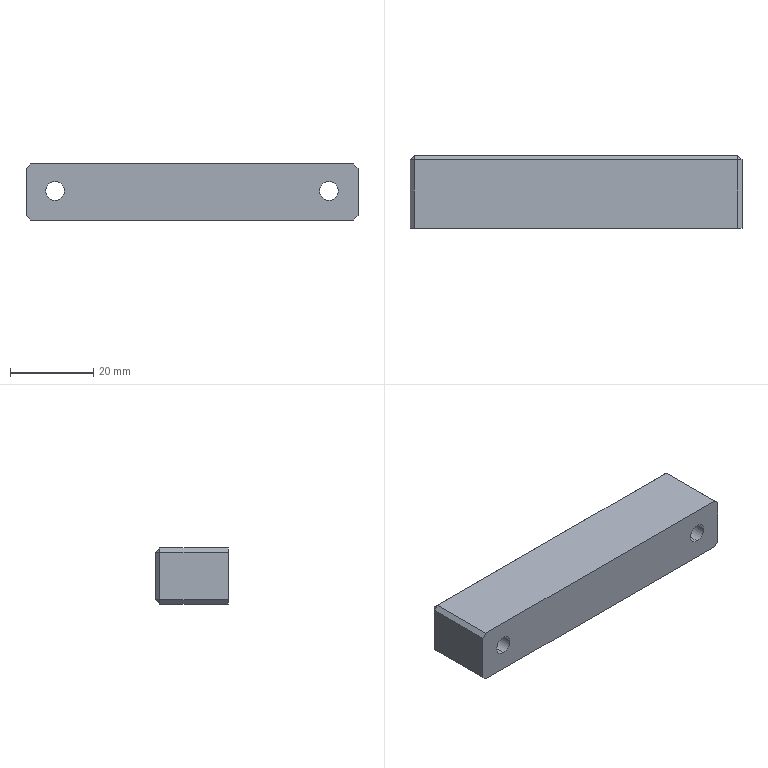Part | STEP file | 229H151426 Default | 1 solid | 28 faces | box 80 x 17.5 x 13.5 mm | volume 17874 mm3 | plane 20 | cylinder 8 | commonest cylinder face diameters 4.5 x4 8 x4
STEP:
#1=CARTESIAN_POINT('',(-33.,3.75,3.));
#2=VERTEX_POINT('',#1);
#3=CARTESIAN_POINT('',(-33.,3.75,11.));
#4=VERTEX_POINT('',#3);
#5=CARTESIAN_POINT('',(-33.,3.75,7.));
#6=DIRECTION('',(0.,1.,0.));
#7=DIRECTION('',(0.,0.,1.));
#8=AXIS2_PLACEMENT_3D('',#5,#6,#7);
#9=CIRCLE('',#8,4.);
#10=EDGE_CURVE('',#2,#4,#9,.T.);
#11=ORIENTED_EDGE('',*,*,#10,.F.);
#12=CARTESIAN_POINT('',(-33.,8.75,3.));
#13=VERTEX_POINT('',#12);
#14=CARTESIAN_POINT('',(-33.,8.75,3.));
#15=DIRECTION('',(0.,1.,0.));
#16=VECTOR('',#15,1000.);
#17=LINE('',#14,#16);
#18=EDGE_CURVE('',#2,#13,#17,.T.);
#19=ORIENTED_EDGE('',*,*,#18,.T.);
#20=CARTESIAN_POINT('',(-33.,8.75,11.));
#21=VERTEX_POINT('',#20);
#22=CARTESIAN_POINT('',(-33.,8.75,7.));
#23=DIRECTION('',(0.,1.,0.));
#24=DIRECTION('',(0.,0.,1.));
#25=AXIS2_PLACEMENT_3D('',#22,#23,#24);
#26=CIRCLE('',#25,4.);
#27=EDGE_CURVE('',#13,#21,#26,.T.);
#28=ORIENTED_EDGE('',*,*,#27,.T.);
#29=CARTESIAN_POINT('',(-33.,8.75,11.));
#30=DIRECTION('',(0.,1.,0.));
#31=VECTOR('',#30,1000.);
#32=LINE('',#29,#31);
#33=EDGE_CURVE('',#4,#21,#32,.T.);
#34=ORIENTED_EDGE('',*,*,#33,.F.);
#35=EDGE_LOOP('',(#11,#19,#28,#34));
#36=FACE_OUTER_BOUND('',#35,.T.);
#37=CARTESIAN_POINT('',(-33.,8.75,7.));
#38=DIRECTION('',(0.,1.,0.));
#39=DIRECTION('',(0.,0.,1.));
#40=AXIS2_PLACEMENT_3D('',#37,#38,#39);
#41=CYLINDRICAL_SURFACE('',#40,4.);
#42=ADVANCED_FACE('',(#36),#41,.F.);
#43=CARTESIAN_POINT('',(-33.,-8.75,4.75));
#44=VERTEX_POINT('',#43);
#45=CARTESIAN_POINT('',(-33.,-8.75,9.25));
#46=VERTEX_POINT('',#45);
#47=CARTESIAN_POINT('',(-33.,-8.75,7.));
#48=DIRECTION('',(0.,1.,0.));
#49=DIRECTION('',(0.,0.,1.));
#50=AXIS2_PLACEMENT_3D('',#47,#48,#49);
#51=CIRCLE('',#50,2.25);
#52=EDGE_CURVE('',#44,#46,#51,.T.);
#53=ORIENTED_EDGE('',*,*,#52,.F.);
#54=CARTESIAN_POINT('',(-33.,3.75,4.75));
#55=VERTEX_POINT('',#54);
#56=CARTESIAN_POINT('',(-33.,8.75,4.75));
#57=DIRECTION('',(0.,1.,0.));
#58=VECTOR('',#57,1000.);
#59=LINE('',#56,#58);
#60=EDGE_CURVE('',#44,#55,#59,.T.);
#61=ORIENTED_EDGE('',*,*,#60,.T.);
#62=CARTESIAN_POINT('',(-33.,3.75,9.25));
#63=VERTEX_POINT('',#62);
#64=CARTESIAN_POINT('',(-33.,3.75,7.));
#65=DIRECTION('',(0.,1.,0.));
#66=DIRECTION('',(0.,0.,1.));
#67=AXIS2_PLACEMENT_3D('',#64,#65,#66);
#68=CIRCLE('',#67,2.25);
#69=EDGE_CURVE('',#55,#63,#68,.T.);
#70=ORIENTED_EDGE('',*,*,#69,.T.);
#71=CARTESIAN_POINT('',(-33.,8.75,9.25));
#72=DIRECTION('',(0.,1.,0.));
#73=VECTOR('',#72,1000.);
#74=LINE('',#71,#73);
#75=EDGE_CURVE('',#46,#63,#74,.T.);
#76=ORIENTED_EDGE('',*,*,#75,.F.);
#77=EDGE_LOOP('',(#53,#61,#70,#76));
#78=FACE_OUTER_BOUND('',#77,.T.);
#79=CARTESIAN_POINT('',(-33.,8.75,7.));
#80=DIRECTION('',(0.,1.,0.));
#81=DIRECTION('',(0.,0.,1.));
#82=AXIS2_PLACEMENT_3D('',#79,#80,#81);
#83=CYLINDRICAL_SURFACE('',#82,2.25);
#84=ADVANCED_FACE('',(#78),#83,.F.);
#85=CARTESIAN_POINT('',(33.,3.75,3.));
#86=VERTEX_POINT('',#85);
#87=CARTESIAN_POINT('',(33.,3.75,11.));
#88=VERTEX_POINT('',#87);
#89=CARTESIAN_POINT('',(33.,3.75,7.));
#90=DIRECTION('',(0.,1.,0.));
#91=DIRECTION('',(0.,0.,1.));
#92=AXIS2_PLACEMENT_3D('',#89,#90,#91);
#93=CIRCLE('',#92,4.);
#94=EDGE_CURVE('',#86,#88,#93,.T.);
#95=ORIENTED_EDGE('',*,*,#94,.F.);
#96=CARTESIAN_POINT('',(33.,8.75,3.));
#97=VERTEX_POINT('',#96);
#98=CARTESIAN_POINT('',(33.,8.75,3.));
#99=DIRECTION('',(0.,1.,0.));
#100=VECTOR('',#99,1000.);
#101=LINE('',#98,#100);
#102=EDGE_CURVE('',#86,#97,#101,.T.);
#103=ORIENTED_EDGE('',*,*,#102,.T.);
#104=CARTESIAN_POINT('',(33.,8.75,11.));
#105=VERTEX_POINT('',#104);
#106=CARTESIAN_POINT('',(33.,8.75,7.));
#107=DIRECTION('',(0.,1.,0.));
#108=DIRECTION('',(0.,0.,1.));
#109=AXIS2_PLACEMENT_3D('',#106,#107,#108);
#110=CIRCLE('',#109,4.);
#111=EDGE_CURVE('',#97,#105,#110,.T.);
#112=ORIENTED_EDGE('',*,*,#111,.T.);
#113=CARTESIAN_POINT('',(33.,8.75,11.));
#114=DIRECTION('',(0.,1.,0.));
#115=VECTOR('',#114,1000.);
#116=LINE('',#113,#115);
#117=EDGE_CURVE('',#88,#105,#116,.T.);
#118=ORIENTED_EDGE('',*,*,#117,.F.);
#119=EDGE_LOOP('',(#95,#103,#112,#118));
#120=FACE_OUTER_BOUND('',#119,.T.);
#121=CARTESIAN_POINT('',(33.,8.75,7.));
#122=DIRECTION('',(0.,1.,0.));
#123=DIRECTION('',(0.,0.,1.));
#124=AXIS2_PLACEMENT_3D('',#121,#122,#123);
#125=CYLINDRICAL_SURFACE('',#124,4.);
#126=ADVANCED_FACE('',(#120),#125,.F.);
#127=CARTESIAN_POINT('',(33.,-8.75,4.75));
#128=VERTEX_POINT('',#127);
#129=CARTESIAN_POINT('',(33.,-8.75,9.25));
#130=VERTEX_POINT('',#129);
#131=CARTESIAN_POINT('',(33.,-8.75,7.));
#132=DIRECTION('',(0.,1.,0.));
#133=DIRECTION('',(0.,0.,1.));
#134=AXIS2_PLACEMENT_3D('',#131,#132,#133);
#135=CIRCLE('',#134,2.25);
#136=EDGE_CURVE('',#128,#130,#135,.T.);
#137=ORIENTED_EDGE('',*,*,#136,.F.);
#138=CARTESIAN_POINT('',(33.,3.75,4.75));
#139=VERTEX_POINT('',#138);
#140=CARTESIAN_POINT('',(33.,8.75,4.75));
#141=DIRECTION('',(0.,1.,0.));
#142=VECTOR('',#141,1000.);
#143=LINE('',#140,#142);
#144=EDGE_CURVE('',#128,#139,#143,.T.);
#145=ORIENTED_EDGE('',*,*,#144,.T.);
#146=CARTESIAN_POINT('',(33.,3.75,9.25));
#147=VERTEX_POINT('',#146);
#148=CARTESIAN_POINT('',(33.,3.75,7.));
#149=DIRECTION('',(0.,1.,0.));
#150=DIRECTION('',(0.,0.,1.));
#151=AXIS2_PLACEMENT_3D('',#148,#149,#150);
#152=CIRCLE('',#151,2.25);
#153=EDGE_CURVE('',#139,#147,#152,.T.);
#154=ORIENTED_EDGE('',*,*,#153,.T.);
#155=CARTESIAN_POINT('',(33.,8.75,9.25));
#156=DIRECTION('',(0.,1.,0.));
#157=VECTOR('',#156,1000.);
#158=LINE('',#155,#157);
#159=EDGE_CURVE('',#130,#147,#158,.T.);
#160=ORIENTED_EDGE('',*,*,#159,.F.);
#161=EDGE_LOOP('',(#137,#145,#154,#160));
#162=FACE_OUTER_BOUND('',#161,.T.);
#163=CARTESIAN_POINT('',(33.,8.75,7.));
#164=DIRECTION('',(0.,1.,0.));
#165=DIRECTION('',(0.,0.,1.));
#166=AXIS2_PLACEMENT_3D('',#163,#164,#165);
#167=CYLINDRICAL_SURFACE('',#166,2.25);
#168=ADVANCED_FACE('',(#162),#167,.F.);
#169=CARTESIAN_POINT('',(40.,-8.75,12.5));
#170=VERTEX_POINT('',#169);
#171=CARTESIAN_POINT('',(40.,-8.75,1.));
#172=VERTEX_POINT('',#171);
#173=CARTESIAN_POINT('',(40.,-8.75,13.5));
#174=DIRECTION('',(0.,0.,-1.));
#175=VECTOR('',#174,1000.);
#176=LINE('',#173,#175);
#177=EDGE_CURVE('',#170,#172,#176,.T.);
#178=ORIENTED_EDGE('',*,*,#177,.T.);
#179=CARTESIAN_POINT('',(40.,7.75,1.));
#180=VERTEX_POINT('',#179);
#181=CARTESIAN_POINT('',(40.,8.75,1.));
#182=DIRECTION('',(0.,1.,0.));
#183=VECTOR('',#182,1000.);
#184=LINE('',#181,#183);
#185=EDGE_CURVE('',#172,#180,#184,.T.);
#186=ORIENTED_EDGE('',*,*,#185,.T.);
#187=CARTESIAN_POINT('',(40.,7.75,12.5));
#188=VERTEX_POINT('',#187);
#189=CARTESIAN_POINT('',(40.,7.75,13.5));
#190=DIRECTION('',(0.,0.,1.));
#191=VECTOR('',#190,1000.);
#192=LINE('',#189,#191);
#193=EDGE_CURVE('',#180,#188,#192,.T.);
#194=ORIENTED_EDGE('',*,*,#193,.T.);
#195=CARTESIAN_POINT('',(40.,-8.75,12.5));
#196=DIRECTION('',(0.,-1.,0.));
#197=VECTOR('',#196,1000.);
#198=LINE('',#195,#197);
#199=EDGE_CURVE('',#188,#170,#198,.T.);
#200=ORIENTED_EDGE('',*,*,#199,.T.);
#201=EDGE_LOOP('',(#178,#186,#194,#200));
#202=FACE_OUTER_BOUND('',#201,.T.);
#203=CARTESIAN_POINT('',(40.,8.75,13.5));
#204=DIRECTION('',(-1.,0.,0.));
#205=DIRECTION('',(0.,0.,1.));
#206=AXIS2_PLACEMENT_3D('',#203,#204,#205);
#207=PLANE('',#206);
#208=ADVANCED_FACE('',(#202),#207,.F.);
#209=CARTESIAN_POINT('',(39.,8.75,12.5));
#210=VERTEX_POINT('',#209);
#211=CARTESIAN_POINT('',(39.,8.75,1.));
#212=VERTEX_POINT('',#211);
#213=CARTESIAN_POINT('',(39.,8.75,13.5));
#214=DIRECTION('',(0.,0.,-1.));
#215=VECTOR('',#214,1000.);
#216=LINE('',#213,#215);
#217=EDGE_CURVE('',#210,#212,#216,.T.);
#218=ORIENTED_EDGE('',*,*,#217,.T.);
#219=CARTESIAN_POINT('',(-39.,8.75,1.));
#220=VERTEX_POINT('',#219);
#221=CARTESIAN_POINT('',(-40.,8.75,1.));
#222=DIRECTION('',(-1.,0.,0.));
#223=VECTOR('',#222,1000.);
#224=LINE('',#221,#223);
#225=EDGE_CURVE('',#212,#220,#224,.T.);
#226=ORIENTED_EDGE('',*,*,#225,.T.);
#227=CARTESIAN_POINT('',(-39.,8.75,12.5));
#228=VERTEX_POINT('',#227);
#229=CARTESIAN_POINT('',(-39.,8.75,13.5));
#230=DIRECTION('',(0.,0.,1.));
#231=VECTOR('',#230,1000.);
#232=LINE('',#229,#231);
#233=EDGE_CURVE('',#220,#228,#232,.T.);
#234=ORIENTED_EDGE('',*,*,#233,.T.);
#235=CARTESIAN_POINT('',(40.,8.75,12.5));
#236=DIRECTION('',(1.,0.,0.));
#237=VECTOR('',#236,1000.);
#238=LINE('',#235,#237);
#239=EDGE_CURVE('',#228,#210,#238,.T.);
#240=ORIENTED_EDGE('',*,*,#239,.T.);
#241=EDGE_LOOP('',(#218,#226,#234,#240));
#242=FACE_OUTER_BOUND('',#241,.T.);
#243=CARTESIAN_POINT('',(-33.,8.75,7.));
#244=DIRECTION('',(0.,1.,0.));
#245=DIRECTION('',(0.,0.,1.));
#246=AXIS2_PLACEMENT_3D('',#243,#244,#245);
#247=CIRCLE('',#246,4.);
#248=EDGE_CURVE('',#21,#13,#247,.T.);
#249=ORIENTED_EDGE('',*,*,#248,.F.);
#250=ORIENTED_EDGE('',*,*,#27,.F.);
#251=EDGE_LOOP('',(#249,#250));
#252=FACE_BOUND('',#251,.T.);
#253=CARTESIAN_POINT('',(33.,8.75,7.));
#254=DIRECTION('',(0.,1.,0.));
#255=DIRECTION('',(0.,0.,1.));
#256=AXIS2_PLACEMENT_3D('',#253,#254,#255);
#257=CIRCLE('',#256,4.);
#258=EDGE_CURVE('',#105,#97,#257,.T.);
#259=ORIENTED_EDGE('',*,*,#258,.F.);
#260=ORIENTED_EDGE('',*,*,#111,.F.);
#261=EDGE_LOOP('',(#259,#260));
#262=FACE_BOUND('',#261,.T.);
#263=CARTESIAN_POINT('',(-40.,8.75,13.5));
#264=DIRECTION('',(0.,-1.,0.));
#265=DIRECTION('',(0.,0.,-1.));
#266=AXIS2_PLACEMENT_3D('',#263,#264,#265);
#267=PLANE('',#266);
#268=ADVANCED_FACE('',(#242,#252,#262),#267,.F.);
#269=CARTESIAN_POINT('',(-40.,-8.75,12.5));
#270=VERTEX_POINT('',#269);
#271=CARTESIAN_POINT('',(-40.,-8.75,1.));
#272=VERTEX_POINT('',#271);
#273=CARTESIAN_POINT('',(-40.,-8.75,13.5));
#274=DIRECTION('',(0.,0.,-1.));
#275=VECTOR('',#274,1000.);
#276=LINE('',#273,#275);
#277=EDGE_CURVE('',#270,#272,#276,.T.);
#278=ORIENTED_EDGE('',*,*,#277,.F.);
#279=CARTESIAN_POINT('',(-40.,7.75,12.5));
#280=VERTEX_POINT('',#279);
#281=CARTESIAN_POINT('',(-40.,8.75,12.5));
#282=DIRECTION('',(0.,1.,0.));
#283=VECTOR('',#282,1000.);
#284=LINE('',#281,#283);
#285=EDGE_CURVE('',#270,#280,#284,.T.);
#286=ORIENTED_EDGE('',*,*,#285,.T.);
#287=CARTESIAN_POINT('',(-40.,7.75,1.));
#288=VERTEX_POINT('',#287);
#289=CARTESIAN_POINT('',(-40.,7.75,13.5));
#290=DIRECTION('',(0.,0.,-1.));
#291=VECTOR('',#290,1000.);
#292=LINE('',#289,#291);
#293=EDGE_CURVE('',#280,#288,#292,.T.);
#294=ORIENTED_EDGE('',*,*,#293,.T.);
#295=CARTESIAN_POINT('',(-40.,8.75,1.));
#296=DIRECTION('',(0.,-1.,0.));
#297=VECTOR('',#296,1000.);
#298=LINE('',#295,#297);
#299=EDGE_CURVE('',#288,#272,#298,.T.);
#300=ORIENTED_EDGE('',*,*,#299,.T.);
#301=EDGE_LOOP('',(#278,#286,#294,#300));
#302=FACE_OUTER_BOUND('',#301,.T.);
#303=CARTESIAN_POINT('',(-40.,8.75,13.5));
#304=DIRECTION('',(1.,0.,0.));
#305=DIRECTION('',(0.,0.,-1.));
#306=AXIS2_PLACEMENT_3D('',#303,#304,#305);
#307=PLANE('',#306);
#308=ADVANCED_FACE('',(#302),#307,.F.);
#309=CARTESIAN_POINT('',(-33.,-8.75,7.));
#310=DIRECTION('',(0.,1.,0.));
#311=DIRECTION('',(0.,0.,1.));
#312=AXIS2_PLACEMENT_3D('',#309,#310,#311);
#313=CIRCLE('',#312,2.25);
#314=EDGE_CURVE('',#46,#44,#313,.T.);
#315=ORIENTED_EDGE('',*,*,#314,.T.);
#316=ORIENTED_EDGE('',*,*,#52,.T.);
#317=EDGE_LOOP('',(#315,#316));
#318=FACE_BOUND('',#317,.T.);
#319=CARTESIAN_POINT('',(33.,-8.75,7.));
#320=DIRECTION('',(0.,1.,0.));
#321=DIRECTION('',(0.,0.,1.));
#322=AXIS2_PLACEMENT_3D('',#319,#320,#321);
#323=CIRCLE('',#322,2.25);
#324=EDGE_CURVE('',#130,#128,#323,.T.);
#325=ORIENTED_EDGE('',*,*,#324,.T.);
#326=ORIENTED_EDGE('',*,*,#136,.T.);
#327=EDGE_LOOP('',(#325,#326));
#328=FACE_BOUND('',#327,.T.);
#329=CARTESIAN_POINT('',(-39.,-8.75,13.5));
#330=VERTEX_POINT('',#329);
#331=CARTESIAN_POINT('',(39.,-8.75,13.5));
#332=VERTEX_POINT('',#331);
#333=CARTESIAN_POINT('',(-40.,-8.75,13.5));
#334=DIRECTION('',(1.,0.,0.));
#335=VECTOR('',#334,1000.);
#336=LINE('',#333,#335);
#337=EDGE_CURVE('',#330,#332,#336,.T.);
#338=ORIENTED_EDGE('',*,*,#337,.F.);
#339=CARTESIAN_POINT('',(-39.,-8.75,13.5));
#340=DIRECTION('',(-0.7071,0.,-0.7071));
#341=VECTOR('',#340,1000.);
#342=LINE('',#339,#341);
#343=EDGE_CURVE('',#330,#270,#342,.T.);
#344=ORIENTED_EDGE('',*,*,#343,.T.);
#345=ORIENTED_EDGE('',*,*,#277,.T.);
#346=CARTESIAN_POINT('',(-39.,-8.75,0.));
#347=VERTEX_POINT('',#346);
#348=CARTESIAN_POINT('',(-40.,-8.75,1.));
#349=DIRECTION('',(0.7071,0.,-0.7071));
#350=VECTOR('',#349,1000.);
#351=LINE('',#348,#350);
#352=EDGE_CURVE('',#272,#347,#351,.T.);
#353=ORIENTED_EDGE('',*,*,#352,.T.);
#354=CARTESIAN_POINT('',(39.,-8.75,0.));
#355=VERTEX_POINT('',#354);
#356=CARTESIAN_POINT('',(-40.,-8.75,0.));
#357=DIRECTION('',(1.,0.,0.));
#358=VECTOR('',#357,1000.);
#359=LINE('',#356,#358);
#360=EDGE_CURVE('',#347,#355,#359,.T.);
#361=ORIENTED_EDGE('',*,*,#360,.T.);
#362=CARTESIAN_POINT('',(40.,-8.75,1.));
#363=DIRECTION('',(0.7071,0.,0.7071));
#364=VECTOR('',#363,1000.);
#365=LINE('',#362,#364);
#366=EDGE_CURVE('',#355,#172,#365,.T.);
#367=ORIENTED_EDGE('',*,*,#366,.T.);
#368=ORIENTED_EDGE('',*,*,#177,.F.);
#369=CARTESIAN_POINT('',(39.,-8.75,13.5));
#370=DIRECTION('',(-0.7071,0.,0.7071));
#371=VECTOR('',#370,1000.);
#372=LINE('',#369,#371);
#373=EDGE_CURVE('',#170,#332,#372,.T.);
#374=ORIENTED_EDGE('',*,*,#373,.T.);
#375=EDGE_LOOP('',(#338,#344,#345,#353,#361,#367,#368,#374));
#376=FACE_OUTER_BOUND('',#375,.T.);
#377=CARTESIAN_POINT('',(-40.,-8.75,13.5));
#378=DIRECTION('',(0.,1.,0.));
#379=DIRECTION('',(0.,0.,1.));
#380=AXIS2_PLACEMENT_3D('',#377,#378,#379);
#381=PLANE('',#380);
#382=ADVANCED_FACE('',(#318,#328,#376),#381,.F.);
#383=CARTESIAN_POINT('',(39.,7.75,13.5));
#384=VERTEX_POINT('',#383);
#385=CARTESIAN_POINT('',(-39.,7.75,13.5));
#386=VERTEX_POINT('',#385);
#387=CARTESIAN_POINT('',(-40.,7.75,13.5));
#388=DIRECTION('',(-1.,0.,0.));
#389=VECTOR('',#388,1000.);
#390=LINE('',#387,#389);
#391=EDGE_CURVE('',#384,#386,#390,.T.);
#392=ORIENTED_EDGE('',*,*,#391,.T.);
#393=CARTESIAN_POINT('',(-39.,-8.75,13.5));
#394=DIRECTION('',(0.,-1.,0.));
#395=VECTOR('',#394,1000.);
#396=LINE('',#393,#395);
#397=EDGE_CURVE('',#386,#330,#396,.T.);
#398=ORIENTED_EDGE('',*,*,#397,.T.);
#399=ORIENTED_EDGE('',*,*,#337,.T.);
#400=CARTESIAN_POINT('',(39.,8.75,13.5));
#401=DIRECTION('',(0.,1.,0.));
#402=VECTOR('',#401,1000.);
#403=LINE('',#400,#402);
#404=EDGE_CURVE('',#332,#384,#403,.T.);
#405=ORIENTED_EDGE('',*,*,#404,.T.);
#406=EDGE_LOOP('',(#392,#398,#399,#405));
#407=FACE_OUTER_BOUND('',#406,.T.);
#408=CARTESIAN_POINT('',(0.,0.,13.5));
#409=DIRECTION('',(0.,0.,1.));
#410=DIRECTION('',(1.,0.,0.));
#411=AXIS2_PLACEMENT_3D('',#408,#409,#410);
#412=PLANE('',#411);
#413=ADVANCED_FACE('',(#407),#412,.T.);
#414=ORIENTED_EDGE('',*,*,#360,.F.);
#415=CARTESIAN_POINT('',(-39.,7.75,0.));
#416=VERTEX_POINT('',#415);
#417=CARTESIAN_POINT('',(-39.,0.,0.));
#418=DIRECTION('',(0.,1.,0.));
#419=VECTOR('',#418,1000.);
#420=LINE('',#417,#419);
#421=EDGE_CURVE('',#347,#416,#420,.T.);
#422=ORIENTED_EDGE('',*,*,#421,.T.);
#423=CARTESIAN_POINT('',(39.,7.75,0.));
#424=VERTEX_POINT('',#423);
#425=CARTESIAN_POINT('',(0.,7.75,0.));
#426=DIRECTION('',(1.,0.,0.));
#427=VECTOR('',#426,1000.);
#428=LINE('',#425,#427);
#429=EDGE_CURVE('',#416,#424,#428,.T.);
#430=ORIENTED_EDGE('',*,*,#429,.T.);
#431=CARTESIAN_POINT('',(39.,0.,0.));
#432=DIRECTION('',(0.,-1.,0.));
#433=VECTOR('',#432,1000.);
#434=LINE('',#431,#433);
#435=EDGE_CURVE('',#424,#355,#434,.T.);
#436=ORIENTED_EDGE('',*,*,#435,.T.);
#437=EDGE_LOOP('',(#414,#422,#430,#436));
#438=FACE_OUTER_BOUND('',#437,.T.);
#439=CARTESIAN_POINT('',(0.,0.,0.));
#440=DIRECTION('',(0.,0.,1.));
#441=DIRECTION('',(1.,0.,0.));
#442=AXIS2_PLACEMENT_3D('',#439,#440,#441);
#443=PLANE('',#442);
#444=ADVANCED_FACE('',(#438),#443,.F.);
#445=ORIENTED_EDGE('',*,*,#144,.F.);
#446=ORIENTED_EDGE('',*,*,#324,.F.);
#447=ORIENTED_EDGE('',*,*,#159,.T.);
#448=CARTESIAN_POINT('',(33.,3.75,7.));
#449=DIRECTION('',(0.,1.,0.));
#450=DIRECTION('',(0.,0.,1.));
#451=AXIS2_PLACEMENT_3D('',#448,#449,#450);
#452=CIRCLE('',#451,2.25);
#453=EDGE_CURVE('',#147,#139,#452,.T.);
#454=ORIENTED_EDGE('',*,*,#453,.T.);
#455=EDGE_LOOP('',(#445,#446,#447,#454));
#456=FACE_OUTER_BOUND('',#455,.T.);
#457=CARTESIAN_POINT('',(33.,8.75,7.));
#458=DIRECTION('',(0.,1.,0.));
#459=DIRECTION('',(0.,0.,1.));
#460=AXIS2_PLACEMENT_3D('',#457,#458,#459);
#461=CYLINDRICAL_SURFACE('',#460,2.25);
#462=ADVANCED_FACE('',(#456),#461,.F.);
#463=ORIENTED_EDGE('',*,*,#453,.F.);
#464=ORIENTED_EDGE('',*,*,#153,.F.);
#465=EDGE_LOOP('',(#463,#464));
#466=FACE_BOUND('',#465,.T.);
#467=CARTESIAN_POINT('',(33.,3.75,7.));
#468=DIRECTION('',(0.,1.,0.));
#469=DIRECTION('',(0.,0.,1.));
#470=AXIS2_PLACEMENT_3D('',#467,#468,#469);
#471=CIRCLE('',#470,4.);
#472=EDGE_CURVE('',#88,#86,#471,.T.);
#473=ORIENTED_EDGE('',*,*,#472,.T.);
#474=ORIENTED_EDGE('',*,*,#94,.T.);
#475=EDGE_LOOP('',(#473,#474));
#476=FACE_OUTER_BOUND('',#475,.T.);
#477=CARTESIAN_POINT('',(35.25,3.75,7.));
#478=DIRECTION('',(0.,-1.,0.));
#479=DIRECTION('',(0.,0.,-1.));
#480=AXIS2_PLACEMENT_3D('',#477,#478,#479);
#481=PLANE('',#480);
#482=ADVANCED_FACE('',(#466,#476),#481,.F.);
#483=ORIENTED_EDGE('',*,*,#102,.F.);
#484=ORIENTED_EDGE('',*,*,#472,.F.);
#485=ORIENTED_EDGE('',*,*,#117,.T.);
#486=ORIENTED_EDGE('',*,*,#258,.T.);
#487=EDGE_LOOP('',(#483,#484,#485,#486));
#488=FACE_OUTER_BOUND('',#487,.T.);
#489=CARTESIAN_POINT('',(33.,8.75,7.));
#490=DIRECTION('',(0.,1.,0.));
#491=DIRECTION('',(0.,0.,1.));
#492=AXIS2_PLACEMENT_3D('',#489,#490,#491);
#493=CYLINDRICAL_SURFACE('',#492,4.);
#494=ADVANCED_FACE('',(#488),#493,.F.);
#495=ORIENTED_EDGE('',*,*,#60,.F.);
#496=ORIENTED_EDGE('',*,*,#314,.F.);
#497=ORIENTED_EDGE('',*,*,#75,.T.);
#498=CARTESIAN_POINT('',(-33.,3.75,7.));
#499=DIRECTION('',(0.,1.,0.));
#500=DIRECTION('',(0.,0.,1.));
#501=AXIS2_PLACEMENT_3D('',#498,#499,#500);
#502=CIRCLE('',#501,2.25);
#503=EDGE_CURVE('',#63,#55,#502,.T.);
#504=ORIENTED_EDGE('',*,*,#503,.T.);
#505=EDGE_LOOP('',(#495,#496,#497,#504));
#506=FACE_OUTER_BOUND('',#505,.T.);
#507=CARTESIAN_POINT('',(-33.,8.75,7.));
#508=DIRECTION('',(0.,1.,0.));
#509=DIRECTION('',(0.,0.,1.));
#510=AXIS2_PLACEMENT_3D('',#507,#508,#509);
#511=CYLINDRICAL_SURFACE('',#510,2.25);
#512=ADVANCED_FACE('',(#506),#511,.F.);
#513=ORIENTED_EDGE('',*,*,#503,.F.);
#514=ORIENTED_EDGE('',*,*,#69,.F.);
#515=EDGE_LOOP('',(#513,#514));
#516=FACE_BOUND('',#515,.T.);
#517=CARTESIAN_POINT('',(-33.,3.75,7.));
#518=DIRECTION('',(0.,1.,0.));
#519=DIRECTION('',(0.,0.,1.));
#520=AXIS2_PLACEMENT_3D('',#517,#518,#519);
#521=CIRCLE('',#520,4.);
#522=EDGE_CURVE('',#4,#2,#521,.T.);
#523=ORIENTED_EDGE('',*,*,#522,.T.);
#524=ORIENTED_EDGE('',*,*,#10,.T.);
#525=EDGE_LOOP('',(#523,#524));
#526=FACE_OUTER_BOUND('',#525,.T.);
#527=CARTESIAN_POINT('',(-30.75,3.75,7.));
#528=DIRECTION('',(0.,-1.,0.));
#529=DIRECTION('',(0.,0.,-1.));
#530=AXIS2_PLACEMENT_3D('',#527,#528,#529);
#531=PLANE('',#530);
#532=ADVANCED_FACE('',(#516,#526),#531,.F.);
#533=ORIENTED_EDGE('',*,*,#18,.F.);
#534=ORIENTED_EDGE('',*,*,#522,.F.);
#535=ORIENTED_EDGE('',*,*,#33,.T.);
#536=ORIENTED_EDGE('',*,*,#248,.T.);
#537=EDGE_LOOP('',(#533,#534,#535,#536));
#538=FACE_OUTER_BOUND('',#537,.T.);
#539=CARTESIAN_POINT('',(-33.,8.75,7.));
#540=DIRECTION('',(0.,1.,0.));
#541=DIRECTION('',(0.,0.,1.));
#542=AXIS2_PLACEMENT_3D('',#539,#540,#541);
#543=CYLINDRICAL_SURFACE('',#542,4.);
#544=ADVANCED_FACE('',(#538),#543,.F.);
#545=ORIENTED_EDGE('',*,*,#373,.F.);
#546=ORIENTED_EDGE('',*,*,#199,.F.);
#547=CARTESIAN_POINT('',(39.5,7.75,13.));
#548=DIRECTION('',(0.7071,0.,-0.7071));
#549=VECTOR('',#548,1000.);
#550=LINE('',#547,#549);
#551=EDGE_CURVE('',#384,#188,#550,.T.);
#552=ORIENTED_EDGE('',*,*,#551,.F.);
#553=ORIENTED_EDGE('',*,*,#404,.F.);
#554=EDGE_LOOP('',(#545,#546,#552,#553));
#555=FACE_OUTER_BOUND('',#554,.T.);
#556=CARTESIAN_POINT('',(39.,0.,13.5));
#557=DIRECTION('',(0.7071,0.,0.7071));
#558=DIRECTION('',(0.,-1.,0.));
#559=AXIS2_PLACEMENT_3D('',#556,#557,#558);
#560=PLANE('',#559);
#561=ADVANCED_FACE('',(#555),#560,.T.);
#562=CARTESIAN_POINT('',(-39.,8.25,13.));
#563=DIRECTION('',(0.,0.7071,-0.7071));
#564=VECTOR('',#563,1000.);
#565=LINE('',#562,#564);
#566=EDGE_CURVE('',#386,#228,#565,.T.);
#567=ORIENTED_EDGE('',*,*,#566,.F.);
#568=ORIENTED_EDGE('',*,*,#391,.F.);
#569=CARTESIAN_POINT('',(39.,8.75,12.5));
#570=DIRECTION('',(0.,-0.7071,0.7071));
#571=VECTOR('',#570,1000.);
#572=LINE('',#569,#571);
#573=EDGE_CURVE('',#210,#384,#572,.T.);
#574=ORIENTED_EDGE('',*,*,#573,.F.);
#575=ORIENTED_EDGE('',*,*,#239,.F.);
#576=EDGE_LOOP('',(#567,#568,#574,#575));
#577=FACE_OUTER_BOUND('',#576,.T.);
#578=CARTESIAN_POINT('',(0.,7.75,13.5));
#579=DIRECTION('',(0.,0.7071,0.7071));
#580=DIRECTION('',(1.,0.,0.));
#581=AXIS2_PLACEMENT_3D('',#578,#579,#580);
#582=PLANE('',#581);
#583=ADVANCED_FACE('',(#577),#582,.T.);
#584=ORIENTED_EDGE('',*,*,#343,.F.);
#585=ORIENTED_EDGE('',*,*,#397,.F.);
#586=CARTESIAN_POINT('',(-40.,7.75,12.5));
#587=DIRECTION('',(0.7071,0.,0.7071));
#588=VECTOR('',#587,1000.);
#589=LINE('',#586,#588);
#590=EDGE_CURVE('',#280,#386,#589,.T.);
#591=ORIENTED_EDGE('',*,*,#590,.F.);
#592=ORIENTED_EDGE('',*,*,#285,.F.);
#593=EDGE_LOOP('',(#584,#585,#591,#592));
#594=FACE_OUTER_BOUND('',#593,.T.);
#595=CARTESIAN_POINT('',(-39.,0.,13.5));
#596=DIRECTION('',(-0.7071,0.,0.7071));
#597=DIRECTION('',(0.,1.,0.));
#598=AXIS2_PLACEMENT_3D('',#595,#596,#597);
#599=PLANE('',#598);
#600=ADVANCED_FACE('',(#594),#599,.T.);
#601=ORIENTED_EDGE('',*,*,#573,.T.);
#602=ORIENTED_EDGE('',*,*,#551,.T.);
#603=CARTESIAN_POINT('',(39.,8.75,12.5));
#604=DIRECTION('',(0.7071,-0.7071,0.));
#605=VECTOR('',#604,1000.);
#606=LINE('',#603,#605);
#607=EDGE_CURVE('',#210,#188,#606,.T.);
#608=ORIENTED_EDGE('',*,*,#607,.F.);
#609=EDGE_LOOP('',(#601,#602,#608));
#610=FACE_OUTER_BOUND('',#609,.T.);
#611=CARTESIAN_POINT('',(39.,8.75,12.5));
#612=DIRECTION('',(0.5774,0.5774,0.5774));
#613=DIRECTION('',(0.7071,0.,-0.7071));
#614=AXIS2_PLACEMENT_3D('',#611,#612,#613);
#615=PLANE('',#614);
#616=ADVANCED_FACE('',(#610),#615,.T.);
#617=ORIENTED_EDGE('',*,*,#590,.T.);
#618=ORIENTED_EDGE('',*,*,#566,.T.);
#619=CARTESIAN_POINT('',(-40.,7.75,12.5));
#620=DIRECTION('',(0.7071,0.7071,0.));
#621=VECTOR('',#620,1000.);
#622=LINE('',#619,#621);
#623=EDGE_CURVE('',#280,#228,#622,.T.);
#624=ORIENTED_EDGE('',*,*,#623,.F.);
#625=EDGE_LOOP('',(#617,#618,#624));
#626=FACE_OUTER_BOUND('',#625,.T.);
#627=CARTESIAN_POINT('',(-40.,7.75,12.5));
#628=DIRECTION('',(-0.5774,0.5774,0.5774));
#629=DIRECTION('',(0.7071,0.,0.7071));
#630=AXIS2_PLACEMENT_3D('',#627,#628,#629);
#631=PLANE('',#630);
#632=ADVANCED_FACE('',(#626),#631,.T.);
#633=ORIENTED_EDGE('',*,*,#366,.F.);
#634=ORIENTED_EDGE('',*,*,#435,.F.);
#635=CARTESIAN_POINT('',(39.,7.75,0.));
#636=DIRECTION('',(-0.7071,0.,-0.7071));
#637=VECTOR('',#636,1000.);
#638=LINE('',#635,#637);
#639=EDGE_CURVE('',#180,#424,#638,.T.);
#640=ORIENTED_EDGE('',*,*,#639,.F.);
#641=ORIENTED_EDGE('',*,*,#185,.F.);
#642=EDGE_LOOP('',(#633,#634,#640,#641));
#643=FACE_OUTER_BOUND('',#642,.T.);
#644=CARTESIAN_POINT('',(40.,8.75,1.));
#645=DIRECTION('',(-0.7071,0.,0.7071));
#646=DIRECTION('',(0.,1.,0.));
#647=AXIS2_PLACEMENT_3D('',#644,#645,#646);
#648=PLANE('',#647);
#649=ADVANCED_FACE('',(#643),#648,.F.);
#650=ORIENTED_EDGE('',*,*,#607,.T.);
#651=ORIENTED_EDGE('',*,*,#193,.F.);
#652=CARTESIAN_POINT('',(39.5,8.25,1.));
#653=DIRECTION('',(0.7071,-0.7071,0.));
#654=VECTOR('',#653,1000.);
#655=LINE('',#652,#654);
#656=EDGE_CURVE('',#212,#180,#655,.T.);
#657=ORIENTED_EDGE('',*,*,#656,.F.);
#658=ORIENTED_EDGE('',*,*,#217,.F.);
#659=EDGE_LOOP('',(#650,#651,#657,#658));
#660=FACE_OUTER_BOUND('',#659,.T.);
#661=CARTESIAN_POINT('',(39.,8.75,13.5));
#662=DIRECTION('',(-0.7071,-0.7071,0.));
#663=DIRECTION('',(0.,0.,-1.));
#664=AXIS2_PLACEMENT_3D('',#661,#662,#663);
#665=PLANE('',#664);
#666=ADVANCED_FACE('',(#660),#665,.F.);
#667=ORIENTED_EDGE('',*,*,#623,.T.);
#668=ORIENTED_EDGE('',*,*,#233,.F.);
#669=CARTESIAN_POINT('',(-39.,8.75,1.));
#670=DIRECTION('',(0.7071,0.7071,0.));
#671=VECTOR('',#670,1000.);
#672=LINE('',#669,#671);
#673=EDGE_CURVE('',#288,#220,#672,.T.);
#674=ORIENTED_EDGE('',*,*,#673,.F.);
#675=ORIENTED_EDGE('',*,*,#293,.F.);
#676=EDGE_LOOP('',(#667,#668,#674,#675));
#677=FACE_OUTER_BOUND('',#676,.T.);
#678=CARTESIAN_POINT('',(-40.,7.75,13.5));
#679=DIRECTION('',(0.7071,-0.7071,0.));
#680=DIRECTION('',(0.,0.,-1.));
#681=AXIS2_PLACEMENT_3D('',#678,#679,#680);
#682=PLANE('',#681);
#683=ADVANCED_FACE('',(#677),#682,.F.);
#684=ORIENTED_EDGE('',*,*,#352,.F.);
#685=ORIENTED_EDGE('',*,*,#299,.F.);
#686=CARTESIAN_POINT('',(-39.5,7.75,0.5));
#687=DIRECTION('',(-0.7071,0.,0.7071));
#688=VECTOR('',#687,1000.);
#689=LINE('',#686,#688);
#690=EDGE_CURVE('',#416,#288,#689,.T.);
#691=ORIENTED_EDGE('',*,*,#690,.F.);
#692=ORIENTED_EDGE('',*,*,#421,.F.);
#693=EDGE_LOOP('',(#684,#685,#691,#692));
#694=FACE_OUTER_BOUND('',#693,.T.);
#695=CARTESIAN_POINT('',(-40.,8.75,1.));
#696=DIRECTION('',(0.7071,0.,0.7071));
#697=DIRECTION('',(0.,-1.,0.));
#698=AXIS2_PLACEMENT_3D('',#695,#696,#697);
#699=PLANE('',#698);
#700=ADVANCED_FACE('',(#694),#699,.F.);
#701=ORIENTED_EDGE('',*,*,#656,.T.);
#702=ORIENTED_EDGE('',*,*,#639,.T.);
#703=CARTESIAN_POINT('',(39.,7.75,0.));
#704=DIRECTION('',(0.,-0.7071,-0.7071));
#705=VECTOR('',#704,1000.);
#706=LINE('',#703,#705);
#707=EDGE_CURVE('',#212,#424,#706,.T.);
#708=ORIENTED_EDGE('',*,*,#707,.F.);
#709=EDGE_LOOP('',(#701,#702,#708));
#710=FACE_OUTER_BOUND('',#709,.T.);
#711=CARTESIAN_POINT('',(39.,7.75,0.));
#712=DIRECTION('',(0.5774,0.5774,-0.5774));
#713=DIRECTION('',(-0.7071,0.,-0.7071));
#714=AXIS2_PLACEMENT_3D('',#711,#712,#713);
#715=PLANE('',#714);
#716=ADVANCED_FACE('',(#710),#715,.T.);
#717=ORIENTED_EDGE('',*,*,#690,.T.);
#718=ORIENTED_EDGE('',*,*,#673,.T.);
#719=CARTESIAN_POINT('',(-39.,8.75,1.));
#720=DIRECTION('',(0.,0.7071,0.7071));
#721=VECTOR('',#720,1000.);
#722=LINE('',#719,#721);
#723=EDGE_CURVE('',#416,#220,#722,.T.);
#724=ORIENTED_EDGE('',*,*,#723,.F.);
#725=EDGE_LOOP('',(#717,#718,#724));
#726=FACE_OUTER_BOUND('',#725,.T.);
#727=CARTESIAN_POINT('',(-39.,8.75,1.));
#728=DIRECTION('',(-0.5774,0.5774,-0.5774));
#729=DIRECTION('',(-0.7071,0.,0.7071));
#730=AXIS2_PLACEMENT_3D('',#727,#728,#729);
#731=PLANE('',#730);
#732=ADVANCED_FACE('',(#726),#731,.T.);
#733=ORIENTED_EDGE('',*,*,#707,.T.);
#734=ORIENTED_EDGE('',*,*,#429,.F.);
#735=ORIENTED_EDGE('',*,*,#723,.T.);
#736=ORIENTED_EDGE('',*,*,#225,.F.);
#737=EDGE_LOOP('',(#733,#734,#735,#736));
#738=FACE_OUTER_BOUND('',#737,.T.);
#739=CARTESIAN_POINT('',(-40.,8.75,1.));
#740=DIRECTION('',(0.,-0.7071,0.7071));
#741=DIRECTION('',(-1.,0.,0.));
#742=AXIS2_PLACEMENT_3D('',#739,#740,#741);
#743=PLANE('',#742);
#744=ADVANCED_FACE('',(#738),#743,.F.);
#745=CLOSED_SHELL('',(#42,#84,#126,#168,#208,#268,#308,#382,#413,#444,#462,#482,#494,#512,#532,#544,#561,#583,#600,#616,#632,#649,#666,#683,#700,#716,#732,#744));
#746=MANIFOLD_SOLID_BREP('',#745);
#747=CARTESIAN_POINT('',(0.,0.,0.));
#748=DIRECTION('',(0.,0.,1.));
#749=DIRECTION('',(1.,0.,0.));
#750=AXIS2_PLACEMENT_3D('',#747,#748,#749);
#751=(LENGTH_UNIT()NAMED_UNIT(*)SI_UNIT(.MILLI.,.METRE.));
#752=UNCERTAINTY_MEASURE_WITH_UNIT(LENGTH_MEASURE(0.00001),#751,'','');
#753=(NAMED_UNIT(*)PLANE_ANGLE_UNIT()SI_UNIT($,.RADIAN.));
#754=(NAMED_UNIT(*)SI_UNIT($,.STERADIAN.)SOLID_ANGLE_UNIT());
#755=(GEOMETRIC_REPRESENTATION_CONTEXT(3)GLOBAL_UNCERTAINTY_ASSIGNED_CONTEXT((#752))GLOBAL_UNIT_ASSIGNED_CONTEXT((#751,#753,#754))REPRESENTATION_CONTEXT('',''));
#756=ADVANCED_BREP_SHAPE_REPRESENTATION('',(#746,#750),#755);